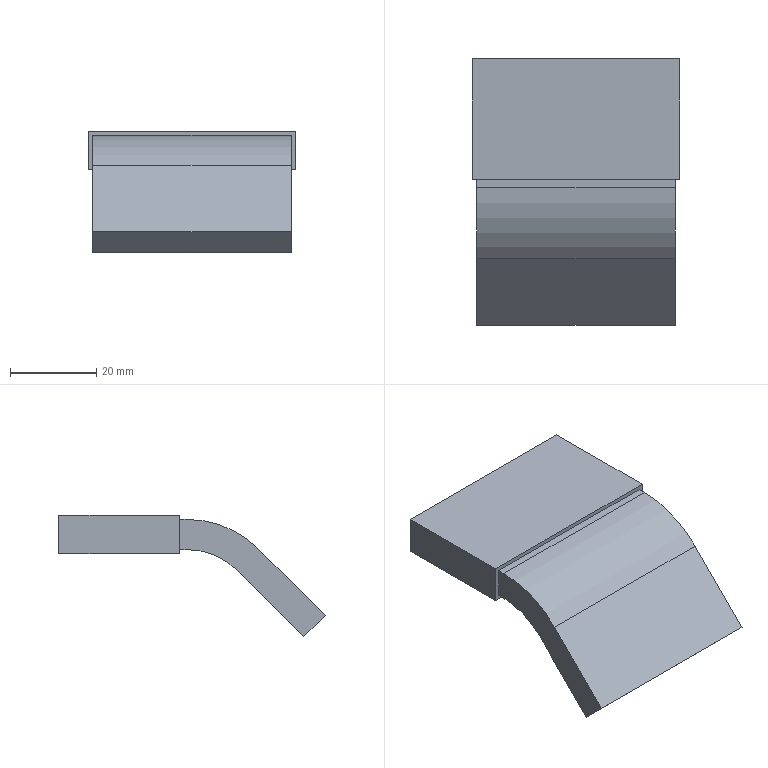Part | NX | features EXTRUDE 2, DATUM_CSYS 1, LINKED_FACE 1, SKETCH 1, UNITE 1 | 1 solid | 15 faces | box 48 x 61.688 x 28.188 mm | volume 24699 mm3 | plane 13 | cylinder 2 | commonest cylinder face diameters 33 x1 47 x1
STEP:
#1=CARTESIAN_POINT('',(24.,-14.,-4.5));
#2=VERTEX_POINT('',#1);
#3=CARTESIAN_POINT('',(24.,14.,-4.5));
#4=VERTEX_POINT('',#3);
#5=CARTESIAN_POINT('',(24.,-14.,-4.5));
#6=DIRECTION('',(0.,1.,0.));
#7=VECTOR('',#6,1000.);
#8=LINE('',#5,#7);
#9=EDGE_CURVE('',#2,#4,#8,.T.);
#10=ORIENTED_EDGE('',*,*,#9,.F.);
#11=CARTESIAN_POINT('',(-24.,-14.,-4.5));
#12=VERTEX_POINT('',#11);
#13=CARTESIAN_POINT('',(-24.,-14.,-4.5));
#14=DIRECTION('',(1.,0.,0.));
#15=VECTOR('',#14,1000.);
#16=LINE('',#13,#15);
#17=EDGE_CURVE('',#12,#2,#16,.T.);
#18=ORIENTED_EDGE('',*,*,#17,.F.);
#19=CARTESIAN_POINT('',(-24.,14.,-4.5));
#20=VERTEX_POINT('',#19);
#21=CARTESIAN_POINT('',(-24.,-14.,-4.5));
#22=DIRECTION('',(0.,1.,0.));
#23=VECTOR('',#22,1000.);
#24=LINE('',#21,#23);
#25=EDGE_CURVE('',#12,#20,#24,.T.);
#26=ORIENTED_EDGE('',*,*,#25,.T.);
#27=CARTESIAN_POINT('',(-24.,14.,-4.5));
#28=DIRECTION('',(1.,0.,0.));
#29=VECTOR('',#28,1000.);
#30=LINE('',#27,#29);
#31=EDGE_CURVE('',#20,#4,#30,.T.);
#32=ORIENTED_EDGE('',*,*,#31,.T.);
#33=EDGE_LOOP('',(#10,#18,#26,#32));
#34=FACE_BOUND('',#33,.T.);
#35=CARTESIAN_POINT('',(-24.,-14.,-4.5));
#36=DIRECTION('',(0.,0.,-1.));
#37=DIRECTION('',(-1.,0.,0.));
#38=AXIS2_PLACEMENT_3D('',#35,#36,#37);
#39=PLANE('',#38);
#40=ADVANCED_FACE('',(#34),#39,.T.);
#41=CARTESIAN_POINT('',(24.,14.,4.5));
#42=VERTEX_POINT('',#41);
#43=CARTESIAN_POINT('',(24.,14.,-4.5));
#44=DIRECTION('',(0.,0.,1.));
#45=VECTOR('',#44,1000.);
#46=LINE('',#43,#45);
#47=EDGE_CURVE('',#4,#42,#46,.T.);
#48=ORIENTED_EDGE('',*,*,#47,.F.);
#49=ORIENTED_EDGE('',*,*,#31,.F.);
#50=CARTESIAN_POINT('',(-24.,14.,4.5));
#51=VERTEX_POINT('',#50);
#52=CARTESIAN_POINT('',(-24.,14.,-4.5));
#53=DIRECTION('',(0.,0.,1.));
#54=VECTOR('',#53,1000.);
#55=LINE('',#52,#54);
#56=EDGE_CURVE('',#20,#51,#55,.T.);
#57=ORIENTED_EDGE('',*,*,#56,.T.);
#58=CARTESIAN_POINT('',(-24.,14.,4.5));
#59=DIRECTION('',(1.,0.,0.));
#60=VECTOR('',#59,1000.);
#61=LINE('',#58,#60);
#62=EDGE_CURVE('',#51,#42,#61,.T.);
#63=ORIENTED_EDGE('',*,*,#62,.T.);
#64=EDGE_LOOP('',(#48,#49,#57,#63));
#65=FACE_BOUND('',#64,.T.);
#66=CARTESIAN_POINT('',(-24.,14.,-4.5));
#67=DIRECTION('',(0.,1.,0.));
#68=DIRECTION('',(0.,0.,1.));
#69=AXIS2_PLACEMENT_3D('',#66,#67,#68);
#70=PLANE('',#69);
#71=ADVANCED_FACE('',(#65),#70,.T.);
#72=CARTESIAN_POINT('',(24.,-14.,4.5));
#73=VERTEX_POINT('',#72);
#74=CARTESIAN_POINT('',(24.,14.,4.5));
#75=DIRECTION('',(0.,-1.,0.));
#76=VECTOR('',#75,1000.);
#77=LINE('',#74,#76);
#78=EDGE_CURVE('',#42,#73,#77,.T.);
#79=ORIENTED_EDGE('',*,*,#78,.F.);
#80=ORIENTED_EDGE('',*,*,#62,.F.);
#81=CARTESIAN_POINT('',(-24.,-14.,4.5));
#82=VERTEX_POINT('',#81);
#83=CARTESIAN_POINT('',(-24.,14.,4.5));
#84=DIRECTION('',(0.,-1.,0.));
#85=VECTOR('',#84,1000.);
#86=LINE('',#83,#85);
#87=EDGE_CURVE('',#51,#82,#86,.T.);
#88=ORIENTED_EDGE('',*,*,#87,.T.);
#89=CARTESIAN_POINT('',(-24.,-14.,4.5));
#90=DIRECTION('',(1.,0.,0.));
#91=VECTOR('',#90,1000.);
#92=LINE('',#89,#91);
#93=EDGE_CURVE('',#82,#73,#92,.T.);
#94=ORIENTED_EDGE('',*,*,#93,.T.);
#95=EDGE_LOOP('',(#79,#80,#88,#94));
#96=FACE_BOUND('',#95,.T.);
#97=CARTESIAN_POINT('',(-24.,14.,4.5));
#98=DIRECTION('',(0.,0.,1.));
#99=DIRECTION('',(1.,0.,0.));
#100=AXIS2_PLACEMENT_3D('',#97,#98,#99);
#101=PLANE('',#100);
#102=ADVANCED_FACE('',(#96),#101,.T.);
#103=CARTESIAN_POINT('',(23.,-14.,-3.5));
#104=VERTEX_POINT('',#103);
#105=CARTESIAN_POINT('',(23.,-14.,3.5));
#106=VERTEX_POINT('',#105);
#107=CARTESIAN_POINT('',(23.,-14.,-3.5));
#108=DIRECTION('',(0.,0.,1.));
#109=VECTOR('',#108,1000.);
#110=LINE('',#107,#109);
#111=EDGE_CURVE('',#104,#106,#110,.T.);
#112=ORIENTED_EDGE('',*,*,#111,.F.);
#113=CARTESIAN_POINT('',(-23.,-14.,-3.5));
#114=VERTEX_POINT('',#113);
#115=CARTESIAN_POINT('',(-23.,-14.,-3.5));
#116=DIRECTION('',(1.,0.,0.));
#117=VECTOR('',#116,1000.);
#118=LINE('',#115,#117);
#119=EDGE_CURVE('',#114,#104,#118,.T.);
#120=ORIENTED_EDGE('',*,*,#119,.F.);
#121=CARTESIAN_POINT('',(-23.,-14.,3.5));
#122=VERTEX_POINT('',#121);
#123=CARTESIAN_POINT('',(-23.,-14.,-3.5));
#124=DIRECTION('',(0.,0.,1.));
#125=VECTOR('',#124,1000.);
#126=LINE('',#123,#125);
#127=EDGE_CURVE('',#114,#122,#126,.T.);
#128=ORIENTED_EDGE('',*,*,#127,.T.);
#129=CARTESIAN_POINT('',(-23.,-14.,3.5));
#130=DIRECTION('',(1.,0.,0.));
#131=VECTOR('',#130,1000.);
#132=LINE('',#129,#131);
#133=EDGE_CURVE('',#122,#106,#132,.T.);
#134=ORIENTED_EDGE('',*,*,#133,.T.);
#135=EDGE_LOOP('',(#112,#120,#128,#134));
#136=FACE_BOUND('',#135,.T.);
#137=CARTESIAN_POINT('',(24.,-14.,3.5));
#138=DIRECTION('',(0.,0.,-1.));
#139=VECTOR('',#138,1000.);
#140=LINE('',#137,#139);
#141=EDGE_CURVE('',#73,#2,#140,.T.);
#142=ORIENTED_EDGE('',*,*,#141,.F.);
#143=ORIENTED_EDGE('',*,*,#93,.F.);
#144=CARTESIAN_POINT('',(-24.,-14.,-3.5));
#145=DIRECTION('',(0.,0.,-1.));
#146=VECTOR('',#145,1000.);
#147=LINE('',#144,#146);
#148=EDGE_CURVE('',#82,#12,#147,.T.);
#149=ORIENTED_EDGE('',*,*,#148,.T.);
#150=ORIENTED_EDGE('',*,*,#17,.T.);
#151=EDGE_LOOP('',(#142,#143,#149,#150));
#152=FACE_BOUND('',#151,.T.);
#153=CARTESIAN_POINT('',(-24.,-14.,3.5));
#154=DIRECTION('',(0.,-1.,0.));
#155=DIRECTION('',(0.,0.,-1.));
#156=AXIS2_PLACEMENT_3D('',#153,#154,#155);
#157=PLANE('',#156);
#158=ADVANCED_FACE('',(#136,#152),#157,.T.);
#159=ORIENTED_EDGE('',*,*,#148,.F.);
#160=ORIENTED_EDGE('',*,*,#87,.F.);
#161=ORIENTED_EDGE('',*,*,#56,.F.);
#162=ORIENTED_EDGE('',*,*,#25,.F.);
#163=EDGE_LOOP('',(#159,#160,#161,#162));
#164=FACE_BOUND('',#163,.T.);
#165=CARTESIAN_POINT('',(-24.,0.,0.));
#166=DIRECTION('',(1.,0.,0.));
#167=DIRECTION('',(0.,0.,-1.));
#168=AXIS2_PLACEMENT_3D('',#165,#166,#167);
#169=PLANE('',#168);
#170=ADVANCED_FACE('',(#164),#169,.F.);
#171=ORIENTED_EDGE('',*,*,#141,.T.);
#172=ORIENTED_EDGE('',*,*,#9,.T.);
#173=ORIENTED_EDGE('',*,*,#47,.T.);
#174=ORIENTED_EDGE('',*,*,#78,.T.);
#175=EDGE_LOOP('',(#171,#172,#173,#174));
#176=FACE_BOUND('',#175,.T.);
#177=CARTESIAN_POINT('',(24.,0.,0.));
#178=DIRECTION('',(1.,0.,0.));
#179=DIRECTION('',(0.,0.,-1.));
#180=AXIS2_PLACEMENT_3D('',#177,#178,#179);
#181=PLANE('',#180);
#182=ADVANCED_FACE('',(#176),#181,.T.);
#183=CARTESIAN_POINT('',(23.,-47.688,-18.738));
#184=VERTEX_POINT('',#183);
#185=CARTESIAN_POINT('',(23.,-42.738,-23.688));
#186=VERTEX_POINT('',#185);
#187=CARTESIAN_POINT('',(23.,-47.688,-18.738));
#188=DIRECTION('',(0.,0.7071,-0.7071));
#189=VECTOR('',#188,1000.);
#190=LINE('',#187,#189);
#191=EDGE_CURVE('',#184,#186,#190,.T.);
#192=ORIENTED_EDGE('',*,*,#191,.F.);
#193=CARTESIAN_POINT('',(-23.,-47.688,-18.738));
#194=VERTEX_POINT('',#193);
#195=CARTESIAN_POINT('',(-23.,-47.688,-18.738));
#196=DIRECTION('',(1.,0.,0.));
#197=VECTOR('',#196,1000.);
#198=LINE('',#195,#197);
#199=EDGE_CURVE('',#194,#184,#198,.T.);
#200=ORIENTED_EDGE('',*,*,#199,.F.);
#201=CARTESIAN_POINT('',(-23.,-42.738,-23.688));
#202=VERTEX_POINT('',#201);
#203=CARTESIAN_POINT('',(-23.,-47.688,-18.738));
#204=DIRECTION('',(0.,0.7071,-0.7071));
#205=VECTOR('',#204,1000.);
#206=LINE('',#203,#205);
#207=EDGE_CURVE('',#194,#202,#206,.T.);
#208=ORIENTED_EDGE('',*,*,#207,.T.);
#209=CARTESIAN_POINT('',(-23.,-42.738,-23.688));
#210=DIRECTION('',(1.,0.,0.));
#211=VECTOR('',#210,1000.);
#212=LINE('',#209,#211);
#213=EDGE_CURVE('',#202,#186,#212,.T.);
#214=ORIENTED_EDGE('',*,*,#213,.T.);
#215=EDGE_LOOP('',(#192,#200,#208,#214));
#216=FACE_BOUND('',#215,.T.);
#217=CARTESIAN_POINT('',(-23.,-47.688,-18.738));
#218=DIRECTION('',(0.,-0.7071,-0.7071));
#219=DIRECTION('',(0.,0.7071,-0.7071));
#220=AXIS2_PLACEMENT_3D('',#217,#218,#219);
#221=PLANE('',#220);
#222=ADVANCED_FACE('',(#216),#221,.T.);
#223=CARTESIAN_POINT('',(23.,-27.383,-8.333));
#224=VERTEX_POINT('',#223);
#225=CARTESIAN_POINT('',(23.,-42.738,-23.688));
#226=DIRECTION('',(0.,0.7071,0.7071));
#227=VECTOR('',#226,1000.);
#228=LINE('',#225,#227);
#229=EDGE_CURVE('',#186,#224,#228,.T.);
#230=ORIENTED_EDGE('',*,*,#229,.F.);
#231=ORIENTED_EDGE('',*,*,#213,.F.);
#232=CARTESIAN_POINT('',(-23.,-27.383,-8.333));
#233=VERTEX_POINT('',#232);
#234=CARTESIAN_POINT('',(-23.,-42.738,-23.688));
#235=DIRECTION('',(0.,0.7071,0.7071));
#236=VECTOR('',#235,1000.);
#237=LINE('',#234,#236);
#238=EDGE_CURVE('',#202,#233,#237,.T.);
#239=ORIENTED_EDGE('',*,*,#238,.T.);
#240=CARTESIAN_POINT('',(-23.,-27.383,-8.333));
#241=DIRECTION('',(1.,0.,0.));
#242=VECTOR('',#241,1000.);
#243=LINE('',#240,#242);
#244=EDGE_CURVE('',#233,#224,#243,.T.);
#245=ORIENTED_EDGE('',*,*,#244,.T.);
#246=EDGE_LOOP('',(#230,#231,#239,#245));
#247=FACE_BOUND('',#246,.T.);
#248=CARTESIAN_POINT('',(-23.,-42.738,-23.688));
#249=DIRECTION('',(0.,0.7071,-0.7071));
#250=DIRECTION('',(0.,0.7071,0.7071));
#251=AXIS2_PLACEMENT_3D('',#248,#249,#250);
#252=PLANE('',#251);
#253=ADVANCED_FACE('',(#247),#252,.T.);
#254=CARTESIAN_POINT('',(23.,-15.716,-3.5));
#255=VERTEX_POINT('',#254);
#256=CARTESIAN_POINT('',(23.,-15.716,-20.));
#257=DIRECTION('',(-1.,0.,0.));
#258=DIRECTION('',(0.,-0.7071,0.7071));
#259=AXIS2_PLACEMENT_3D('',#256,#257,#258);
#260=CIRCLE('',#259,16.5);
#261=EDGE_CURVE('',#224,#255,#260,.T.);
#262=ORIENTED_EDGE('',*,*,#261,.F.);
#263=ORIENTED_EDGE('',*,*,#244,.F.);
#264=CARTESIAN_POINT('',(-23.,-15.716,-3.5));
#265=VERTEX_POINT('',#264);
#266=CARTESIAN_POINT('',(-23.,-15.716,-20.));
#267=DIRECTION('',(-1.,0.,0.));
#268=DIRECTION('',(0.,-0.7071,0.7071));
#269=AXIS2_PLACEMENT_3D('',#266,#267,#268);
#270=CIRCLE('',#269,16.5);
#271=EDGE_CURVE('',#233,#265,#270,.T.);
#272=ORIENTED_EDGE('',*,*,#271,.T.);
#273=CARTESIAN_POINT('',(-23.,-15.716,-3.5));
#274=DIRECTION('',(1.,0.,0.));
#275=VECTOR('',#274,1000.);
#276=LINE('',#273,#275);
#277=EDGE_CURVE('',#265,#255,#276,.T.);
#278=ORIENTED_EDGE('',*,*,#277,.T.);
#279=EDGE_LOOP('',(#262,#263,#272,#278));
#280=FACE_BOUND('',#279,.T.);
#281=CARTESIAN_POINT('',(-23.,-15.716,-20.));
#282=DIRECTION('',(1.,0.,0.));
#283=DIRECTION('',(0.,0.,-1.));
#284=AXIS2_PLACEMENT_3D('',#281,#282,#283);
#285=CYLINDRICAL_SURFACE('',#284,16.5);
#286=ADVANCED_FACE('',(#280),#285,.F.);
#287=CARTESIAN_POINT('',(23.,-15.716,-3.5));
#288=DIRECTION('',(0.,1.,0.));
#289=VECTOR('',#288,1000.);
#290=LINE('',#287,#289);
#291=EDGE_CURVE('',#255,#104,#290,.T.);
#292=ORIENTED_EDGE('',*,*,#291,.F.);
#293=ORIENTED_EDGE('',*,*,#277,.F.);
#294=CARTESIAN_POINT('',(-23.,-15.716,-3.5));
#295=DIRECTION('',(0.,1.,0.));
#296=VECTOR('',#295,1000.);
#297=LINE('',#294,#296);
#298=EDGE_CURVE('',#265,#114,#297,.T.);
#299=ORIENTED_EDGE('',*,*,#298,.T.);
#300=ORIENTED_EDGE('',*,*,#119,.T.);
#301=EDGE_LOOP('',(#292,#293,#299,#300));
#302=FACE_BOUND('',#301,.T.);
#303=CARTESIAN_POINT('',(-23.,-15.716,-3.5));
#304=DIRECTION('',(0.,0.,-1.));
#305=DIRECTION('',(-1.,0.,0.));
#306=AXIS2_PLACEMENT_3D('',#303,#304,#305);
#307=PLANE('',#306);
#308=ADVANCED_FACE('',(#302),#307,.T.);
#309=CARTESIAN_POINT('',(23.,-15.716,3.5));
#310=VERTEX_POINT('',#309);
#311=CARTESIAN_POINT('',(23.,-14.,3.5));
#312=DIRECTION('',(0.,-1.,0.));
#313=VECTOR('',#312,1000.);
#314=LINE('',#311,#313);
#315=EDGE_CURVE('',#106,#310,#314,.T.);
#316=ORIENTED_EDGE('',*,*,#315,.F.);
#317=ORIENTED_EDGE('',*,*,#133,.F.);
#318=CARTESIAN_POINT('',(-23.,-15.716,3.5));
#319=VERTEX_POINT('',#318);
#320=CARTESIAN_POINT('',(-23.,-14.,3.5));
#321=DIRECTION('',(0.,-1.,0.));
#322=VECTOR('',#321,1000.);
#323=LINE('',#320,#322);
#324=EDGE_CURVE('',#122,#319,#323,.T.);
#325=ORIENTED_EDGE('',*,*,#324,.T.);
#326=CARTESIAN_POINT('',(-23.,-15.716,3.5));
#327=DIRECTION('',(1.,0.,0.));
#328=VECTOR('',#327,1000.);
#329=LINE('',#326,#328);
#330=EDGE_CURVE('',#319,#310,#329,.T.);
#331=ORIENTED_EDGE('',*,*,#330,.T.);
#332=EDGE_LOOP('',(#316,#317,#325,#331));
#333=FACE_BOUND('',#332,.T.);
#334=CARTESIAN_POINT('',(-23.,-14.,3.5));
#335=DIRECTION('',(0.,0.,1.));
#336=DIRECTION('',(1.,0.,0.));
#337=AXIS2_PLACEMENT_3D('',#334,#335,#336);
#338=PLANE('',#337);
#339=ADVANCED_FACE('',(#333),#338,.T.);
#340=CARTESIAN_POINT('',(23.,-32.333,-3.383));
#341=VERTEX_POINT('',#340);
#342=CARTESIAN_POINT('',(23.,-15.716,-20.));
#343=DIRECTION('',(1.,0.,0.));
#344=DIRECTION('',(0.,0.,1.));
#345=AXIS2_PLACEMENT_3D('',#342,#343,#344);
#346=CIRCLE('',#345,23.5);
#347=EDGE_CURVE('',#310,#341,#346,.T.);
#348=ORIENTED_EDGE('',*,*,#347,.F.);
#349=ORIENTED_EDGE('',*,*,#330,.F.);
#350=CARTESIAN_POINT('',(-23.,-32.333,-3.383));
#351=VERTEX_POINT('',#350);
#352=CARTESIAN_POINT('',(-23.,-15.716,-20.));
#353=DIRECTION('',(1.,0.,0.));
#354=DIRECTION('',(0.,0.,1.));
#355=AXIS2_PLACEMENT_3D('',#352,#353,#354);
#356=CIRCLE('',#355,23.5);
#357=EDGE_CURVE('',#319,#351,#356,.T.);
#358=ORIENTED_EDGE('',*,*,#357,.T.);
#359=CARTESIAN_POINT('',(-23.,-32.333,-3.383));
#360=DIRECTION('',(1.,0.,0.));
#361=VECTOR('',#360,1000.);
#362=LINE('',#359,#361);
#363=EDGE_CURVE('',#351,#341,#362,.T.);
#364=ORIENTED_EDGE('',*,*,#363,.T.);
#365=EDGE_LOOP('',(#348,#349,#358,#364));
#366=FACE_BOUND('',#365,.T.);
#367=CARTESIAN_POINT('',(-23.,-15.716,-20.));
#368=DIRECTION('',(1.,0.,0.));
#369=DIRECTION('',(0.,0.,-1.));
#370=AXIS2_PLACEMENT_3D('',#367,#368,#369);
#371=CYLINDRICAL_SURFACE('',#370,23.5);
#372=ADVANCED_FACE('',(#366),#371,.T.);
#373=CARTESIAN_POINT('',(23.,-32.333,-3.383));
#374=DIRECTION('',(0.,-0.7071,-0.7071));
#375=VECTOR('',#374,1000.);
#376=LINE('',#373,#375);
#377=EDGE_CURVE('',#341,#184,#376,.T.);
#378=ORIENTED_EDGE('',*,*,#377,.F.);
#379=ORIENTED_EDGE('',*,*,#363,.F.);
#380=CARTESIAN_POINT('',(-23.,-32.333,-3.383));
#381=DIRECTION('',(0.,-0.7071,-0.7071));
#382=VECTOR('',#381,1000.);
#383=LINE('',#380,#382);
#384=EDGE_CURVE('',#351,#194,#383,.T.);
#385=ORIENTED_EDGE('',*,*,#384,.T.);
#386=ORIENTED_EDGE('',*,*,#199,.T.);
#387=EDGE_LOOP('',(#378,#379,#385,#386));
#388=FACE_BOUND('',#387,.T.);
#389=CARTESIAN_POINT('',(-23.,-32.333,-3.383));
#390=DIRECTION('',(0.,-0.7071,0.7071));
#391=DIRECTION('',(0.,-0.7071,-0.7071));
#392=AXIS2_PLACEMENT_3D('',#389,#390,#391);
#393=PLANE('',#392);
#394=ADVANCED_FACE('',(#388),#393,.T.);
#395=ORIENTED_EDGE('',*,*,#207,.F.);
#396=ORIENTED_EDGE('',*,*,#384,.F.);
#397=ORIENTED_EDGE('',*,*,#357,.F.);
#398=ORIENTED_EDGE('',*,*,#324,.F.);
#399=ORIENTED_EDGE('',*,*,#127,.F.);
#400=ORIENTED_EDGE('',*,*,#298,.F.);
#401=ORIENTED_EDGE('',*,*,#271,.F.);
#402=ORIENTED_EDGE('',*,*,#238,.F.);
#403=EDGE_LOOP('',(#395,#396,#397,#398,#399,#400,#401,#402));
#404=FACE_BOUND('',#403,.T.);
#405=CARTESIAN_POINT('',(-23.,-15.716,-20.));
#406=DIRECTION('',(-1.,0.,0.));
#407=DIRECTION('',(0.,0.,1.));
#408=AXIS2_PLACEMENT_3D('',#405,#406,#407);
#409=PLANE('',#408);
#410=ADVANCED_FACE('',(#404),#409,.T.);
#411=ORIENTED_EDGE('',*,*,#191,.T.);
#412=ORIENTED_EDGE('',*,*,#229,.T.);
#413=ORIENTED_EDGE('',*,*,#261,.T.);
#414=ORIENTED_EDGE('',*,*,#291,.T.);
#415=ORIENTED_EDGE('',*,*,#111,.T.);
#416=ORIENTED_EDGE('',*,*,#315,.T.);
#417=ORIENTED_EDGE('',*,*,#347,.T.);
#418=ORIENTED_EDGE('',*,*,#377,.T.);
#419=EDGE_LOOP('',(#411,#412,#413,#414,#415,#416,#417,#418));
#420=FACE_BOUND('',#419,.T.);
#421=CARTESIAN_POINT('',(23.,-15.716,-20.));
#422=DIRECTION('',(-1.,0.,0.));
#423=DIRECTION('',(0.,0.,1.));
#424=AXIS2_PLACEMENT_3D('',#421,#422,#423);
#425=PLANE('',#424);
#426=ADVANCED_FACE('',(#420),#425,.F.);
#427=CLOSED_SHELL('',(#40,#71,#102,#158,#170,#182,#222,#253,#286,#308,#339,#372,#394,#410,#426));
#428=MANIFOLD_SOLID_BREP('',#427);
#429=(LENGTH_UNIT()NAMED_UNIT(*)SI_UNIT(.MILLI.,.METRE.));
#430=UNCERTAINTY_MEASURE_WITH_UNIT(LENGTH_MEASURE(0.00001),#429,'','');
#431=(NAMED_UNIT(*)PLANE_ANGLE_UNIT()SI_UNIT($,.RADIAN.));
#432=(NAMED_UNIT(*)SI_UNIT($,.STERADIAN.)SOLID_ANGLE_UNIT());
#433=(GEOMETRIC_REPRESENTATION_CONTEXT(3)GLOBAL_UNCERTAINTY_ASSIGNED_CONTEXT((#430))GLOBAL_UNIT_ASSIGNED_CONTEXT((#429,#431,#432))REPRESENTATION_CONTEXT('',''));
#434=ADVANCED_BREP_SHAPE_REPRESENTATION('',(#428),#433);